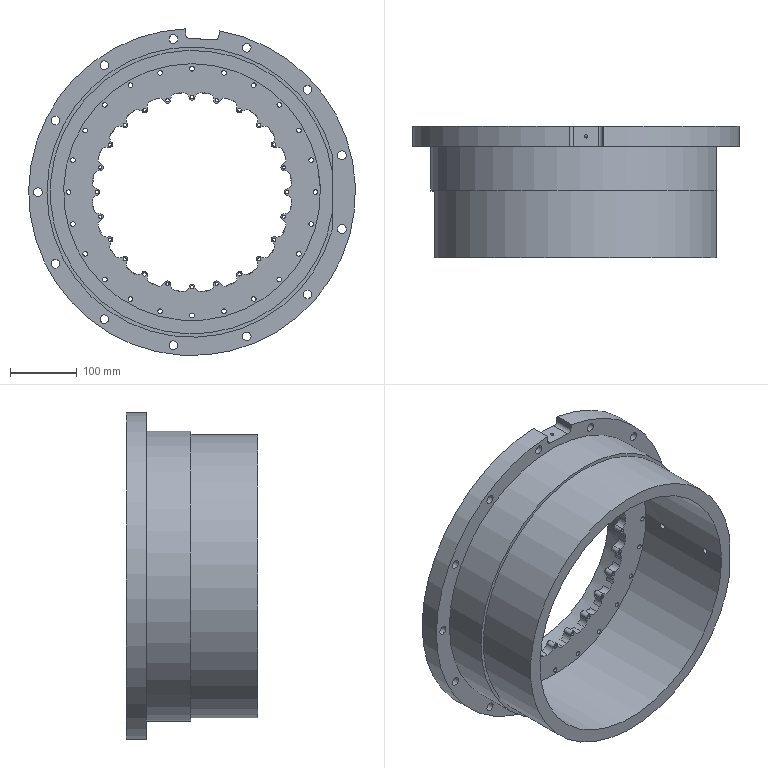Part | STEP file | Outer housing | 1 solid | 330 faces | box 490 x 197 x 489.832 mm | volume 8337866 mm3 | cylinder 202 | plane 70 | cone 58 | commonest cylinder face diameters 20 x61 4.917 x47 7 x24 9 x24 15 x24 13 x13